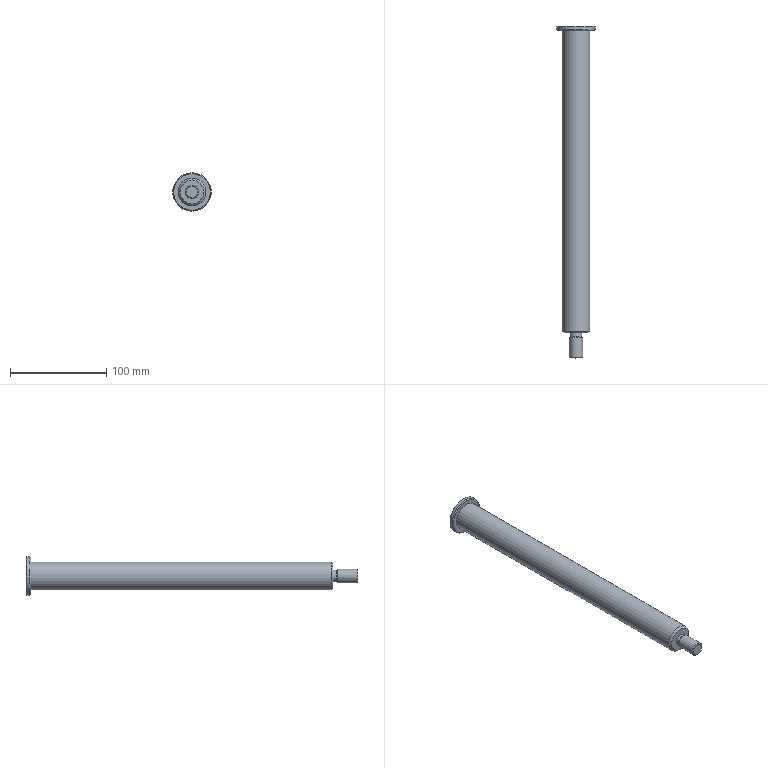Part | STEP file | HL4GZ-1.862.565 swing arm short shaft | 1 solid | 13 faces | box 40 x 345 x 40 mm | volume 217186 mm3 | cone 5 | plane 4 | cylinder 4 | commonest cylinder face diameters 12 x1 14 x1 29 x1 40 x1
STEP:
#1=CARTESIAN_POINT('',(0.,0.,0.));
#2=DIRECTION('',(0.,0.,1.));
#3=DIRECTION('',(1.,0.,0.));
#4=AXIS2_PLACEMENT_3D('',#1,#2,#3);
#5=CARTESIAN_POINT('',(1626.526,-17.,-146.534));
#6=VERTEX_POINT('',#5);
#7=CARTESIAN_POINT('',(1631.,-17.,-165.));
#8=DIRECTION('',(0.,-1.,0.));
#9=DIRECTION('',(0.2355,0.,-0.9719));
#10=AXIS2_PLACEMENT_3D('',#7,#8,#9);
#11=CIRCLE('',#10,19.);
#12=CARTESIAN_POINT('',(1631.,-17.,-165.));
#13=DIRECTION('',(0.,1.,0.));
#14=DIRECTION('',(-0.2355,0.,0.9719));
#15=AXIS2_PLACEMENT_3D('',#12,#13,#14);
#16=PLANE('',#15);
#17=CARTESIAN_POINT('',(-19.,0.));
#18=CARTESIAN_POINT('',(-19.,32.909));
#19=CARTESIAN_POINT('',(9.5,16.454));
#20=CARTESIAN_POINT('',(38.,0.));
#21=CARTESIAN_POINT('',(9.5,-16.454));
#22=CARTESIAN_POINT('',(-19.,-32.909));
#23=CARTESIAN_POINT('',(-19.,0.));
#24=(BOUNDED_CURVE()B_SPLINE_CURVE(2,(#17,#18,#19,#20,#21,#22,#23),.UNSPECIFIED.,.T.,.F.)B_SPLINE_CURVE_WITH_KNOTS((1,2,2,2,2,1),(-2.094,0.,2.094,4.189,6.283,8.378),.UNSPECIFIED.)CURVE()GEOMETRIC_REPRESENTATION_ITEM()RATIONAL_B_SPLINE_CURVE((1.,0.5,1.,0.5,1.,0.5,1.))REPRESENTATION_ITEM(''));
#25=(GEOMETRIC_REPRESENTATION_CONTEXT(2)PARAMETRIC_REPRESENTATION_CONTEXT()REPRESENTATION_CONTEXT('',''));
#26=DEFINITIONAL_REPRESENTATION('',(#24),#25);
#27=PCURVE('',#16,#26);
#28=CARTESIAN_POINT('',(1631.,-17.5,-165.));
#29=DIRECTION('',(0.,-1.,0.));
#30=DIRECTION('',(0.2355,0.,-0.9719));
#31=AXIS2_PLACEMENT_3D('',#28,#29,#30);
#32=CONICAL_SURFACE('',#31,19.5,0.7854);
#33=CARTESIAN_POINT('',(0.,-0.5));
#34=DIRECTION('',(1.,0.));
#35=VECTOR('',#34,1.);
#36=LINE('',#33,#35);
#37=(GEOMETRIC_REPRESENTATION_CONTEXT(2)PARAMETRIC_REPRESENTATION_CONTEXT()REPRESENTATION_CONTEXT('',''));
#38=DEFINITIONAL_REPRESENTATION('',(#36),#37);
#39=PCURVE('',#32,#38);
#40=SURFACE_CURVE('',#11,(#27,#39),.PCURVE_S1.);
#41=EDGE_CURVE('',#6,#6,#40,.T.);
#42=ORIENTED_EDGE('',*,*,#41,.F.);
#43=EDGE_LOOP('',(#42));
#44=FACE_BOUND('',#43,.T.);
#45=ADVANCED_FACE('',(#44),#16,.T.);
#46=ORIENTED_EDGE('',*,*,#41,.T.);
#47=CARTESIAN_POINT('',(1626.29,-18.,-145.562));
#48=VERTEX_POINT('',#47);
#49=CARTESIAN_POINT('',(1626.526,-17.,-146.534));
#50=CARTESIAN_POINT('',(1626.29,-18.,-145.562));
#51=B_SPLINE_CURVE_WITH_KNOTS('',1,(#49,#50),.UNSPECIFIED.,.F.,.F.,(2,2),(-0.7071,0.7071),.PIECEWISE_BEZIER_KNOTS.);
#52=CARTESIAN_POINT('',(9.425,0.));
#53=DIRECTION('',(0.,1.));
#54=VECTOR('',#53,1.);
#55=LINE('',#52,#54);
#56=(GEOMETRIC_REPRESENTATION_CONTEXT(2)PARAMETRIC_REPRESENTATION_CONTEXT()REPRESENTATION_CONTEXT('',''));
#57=DEFINITIONAL_REPRESENTATION('',(#55),#56);
#58=PCURVE('',#32,#57);
#59=CARTESIAN_POINT('',(3.142,0.));
#60=DIRECTION('',(0.,1.));
#61=VECTOR('',#60,1.);
#62=LINE('',#59,#61);
#63=(GEOMETRIC_REPRESENTATION_CONTEXT(2)PARAMETRIC_REPRESENTATION_CONTEXT()REPRESENTATION_CONTEXT('',''));
#64=DEFINITIONAL_REPRESENTATION('',(#62),#63);
#65=PCURVE('',#32,#64);
#66=SEAM_CURVE('',#51,(#58,#65),.PCURVE_S1.);
#67=EDGE_CURVE('',#6,#48,#66,.T.);
#68=ORIENTED_EDGE('',*,*,#67,.T.);
#69=CARTESIAN_POINT('',(1631.,-18.,-165.));
#70=DIRECTION('',(0.,1.,0.));
#71=DIRECTION('',(0.2355,0.,-0.9719));
#72=AXIS2_PLACEMENT_3D('',#69,#70,#71);
#73=CIRCLE('',#72,20.);
#74=CARTESIAN_POINT('',(12.566,0.5));
#75=DIRECTION('',(-1.,0.));
#76=VECTOR('',#75,1.);
#77=LINE('',#74,#76);
#78=(GEOMETRIC_REPRESENTATION_CONTEXT(2)PARAMETRIC_REPRESENTATION_CONTEXT()REPRESENTATION_CONTEXT('',''));
#79=DEFINITIONAL_REPRESENTATION('',(#77),#78);
#80=PCURVE('',#32,#79);
#81=CARTESIAN_POINT('',(1631.,-22.,-165.));
#82=DIRECTION('',(0.,1.,0.));
#83=DIRECTION('',(0.2355,0.,-0.9719));
#84=AXIS2_PLACEMENT_3D('',#81,#82,#83);
#85=CYLINDRICAL_SURFACE('',#84,20.);
#86=CARTESIAN_POINT('',(0.,4.));
#87=DIRECTION('',(1.,0.));
#88=VECTOR('',#87,1.);
#89=LINE('',#86,#88);
#90=(GEOMETRIC_REPRESENTATION_CONTEXT(2)PARAMETRIC_REPRESENTATION_CONTEXT()REPRESENTATION_CONTEXT('',''));
#91=DEFINITIONAL_REPRESENTATION('',(#89),#90);
#92=PCURVE('',#85,#91);
#93=SURFACE_CURVE('',#73,(#80,#92),.PCURVE_S1.);
#94=EDGE_CURVE('',#48,#48,#93,.T.);
#95=ORIENTED_EDGE('',*,*,#94,.T.);
#96=ORIENTED_EDGE('',*,*,#67,.F.);
#97=EDGE_LOOP('',(#46,#68,#95,#96));
#98=FACE_BOUND('',#97,.T.);
#99=ADVANCED_FACE('',(#98),#32,.T.);
#100=ORIENTED_EDGE('',*,*,#94,.F.);
#101=CARTESIAN_POINT('',(1626.29,-21.,-145.562));
#102=VERTEX_POINT('',#101);
#103=CARTESIAN_POINT('',(1626.29,-21.,-145.562));
#104=CARTESIAN_POINT('',(1626.29,-18.,-145.562));
#105=B_SPLINE_CURVE_WITH_KNOTS('',1,(#103,#104),.UNSPECIFIED.,.F.,.F.,(2,2),(1.,4.),.PIECEWISE_BEZIER_KNOTS.);
#106=CARTESIAN_POINT('',(3.142,0.));
#107=DIRECTION('',(0.,1.));
#108=VECTOR('',#107,1.);
#109=LINE('',#106,#108);
#110=(GEOMETRIC_REPRESENTATION_CONTEXT(2)PARAMETRIC_REPRESENTATION_CONTEXT()REPRESENTATION_CONTEXT('',''));
#111=DEFINITIONAL_REPRESENTATION('',(#109),#110);
#112=PCURVE('',#85,#111);
#113=CARTESIAN_POINT('',(9.425,0.));
#114=DIRECTION('',(0.,1.));
#115=VECTOR('',#114,1.);
#116=LINE('',#113,#115);
#117=(GEOMETRIC_REPRESENTATION_CONTEXT(2)PARAMETRIC_REPRESENTATION_CONTEXT()REPRESENTATION_CONTEXT('',''));
#118=DEFINITIONAL_REPRESENTATION('',(#116),#117);
#119=PCURVE('',#85,#118);
#120=SEAM_CURVE('',#105,(#112,#119),.PCURVE_S1.);
#121=EDGE_CURVE('',#102,#48,#120,.T.);
#122=ORIENTED_EDGE('',*,*,#121,.F.);
#123=CARTESIAN_POINT('',(1631.,-21.,-165.));
#124=DIRECTION('',(0.,-1.,0.));
#125=DIRECTION('',(0.2355,0.,-0.9719));
#126=AXIS2_PLACEMENT_3D('',#123,#124,#125);
#127=CIRCLE('',#126,20.);
#128=CARTESIAN_POINT('',(12.566,1.));
#129=DIRECTION('',(-1.,0.));
#130=VECTOR('',#129,1.);
#131=LINE('',#128,#130);
#132=(GEOMETRIC_REPRESENTATION_CONTEXT(2)PARAMETRIC_REPRESENTATION_CONTEXT()REPRESENTATION_CONTEXT('',''));
#133=DEFINITIONAL_REPRESENTATION('',(#131),#132);
#134=PCURVE('',#85,#133);
#135=CARTESIAN_POINT('',(1631.,-21.5,-165.));
#136=DIRECTION('',(0.,1.,0.));
#137=DIRECTION('',(0.2355,0.,-0.9719));
#138=AXIS2_PLACEMENT_3D('',#135,#136,#137);
#139=CONICAL_SURFACE('',#138,19.5,0.7854);
#140=CARTESIAN_POINT('',(12.566,0.5));
#141=DIRECTION('',(-1.,0.));
#142=VECTOR('',#141,1.);
#143=LINE('',#140,#142);
#144=(GEOMETRIC_REPRESENTATION_CONTEXT(2)PARAMETRIC_REPRESENTATION_CONTEXT()REPRESENTATION_CONTEXT('',''));
#145=DEFINITIONAL_REPRESENTATION('',(#143),#144);
#146=PCURVE('',#139,#145);
#147=SURFACE_CURVE('',#127,(#134,#146),.PCURVE_S1.);
#148=EDGE_CURVE('',#102,#102,#147,.T.);
#149=ORIENTED_EDGE('',*,*,#148,.F.);
#150=ORIENTED_EDGE('',*,*,#121,.T.);
#151=EDGE_LOOP('',(#100,#122,#149,#150));
#152=FACE_BOUND('',#151,.T.);
#153=ADVANCED_FACE('',(#152),#85,.T.);
#154=CARTESIAN_POINT('',(1626.526,-22.,-146.534));
#155=VERTEX_POINT('',#154);
#156=CARTESIAN_POINT('',(1631.,-22.,-165.));
#157=DIRECTION('',(0.,1.,0.));
#158=DIRECTION('',(0.2355,0.,-0.9719));
#159=AXIS2_PLACEMENT_3D('',#156,#157,#158);
#160=CIRCLE('',#159,19.);
#161=CARTESIAN_POINT('',(0.,-0.5));
#162=DIRECTION('',(1.,0.));
#163=VECTOR('',#162,1.);
#164=LINE('',#161,#163);
#165=(GEOMETRIC_REPRESENTATION_CONTEXT(2)PARAMETRIC_REPRESENTATION_CONTEXT()REPRESENTATION_CONTEXT('',''));
#166=DEFINITIONAL_REPRESENTATION('',(#164),#165);
#167=PCURVE('',#139,#166);
#168=CARTESIAN_POINT('',(1631.,-22.,-165.));
#169=DIRECTION('',(0.,1.,0.));
#170=DIRECTION('',(-0.2355,0.,0.9719));
#171=AXIS2_PLACEMENT_3D('',#168,#169,#170);
#172=PLANE('',#171);
#173=CARTESIAN_POINT('',(0.,0.));
#174=DIRECTION('',(-1.,0.));
#175=AXIS2_PLACEMENT_2D('',#173,#174);
#176=CIRCLE('',#175,19.);
#177=(GEOMETRIC_REPRESENTATION_CONTEXT(2)PARAMETRIC_REPRESENTATION_CONTEXT()REPRESENTATION_CONTEXT('',''));
#178=DEFINITIONAL_REPRESENTATION('',(#176),#177);
#179=PCURVE('',#172,#178);
#180=SURFACE_CURVE('',#160,(#167,#179),.PCURVE_S1.);
#181=EDGE_CURVE('',#155,#155,#180,.T.);
#182=ORIENTED_EDGE('',*,*,#181,.T.);
#183=CARTESIAN_POINT('',(1626.526,-22.,-146.534));
#184=CARTESIAN_POINT('',(1626.29,-21.,-145.562));
#185=B_SPLINE_CURVE_WITH_KNOTS('',1,(#183,#184),.UNSPECIFIED.,.F.,.F.,(2,2),(-0.7071,0.7071),.PIECEWISE_BEZIER_KNOTS.);
#186=CARTESIAN_POINT('',(9.425,0.));
#187=DIRECTION('',(0.,1.));
#188=VECTOR('',#187,1.);
#189=LINE('',#186,#188);
#190=(GEOMETRIC_REPRESENTATION_CONTEXT(2)PARAMETRIC_REPRESENTATION_CONTEXT()REPRESENTATION_CONTEXT('',''));
#191=DEFINITIONAL_REPRESENTATION('',(#189),#190);
#192=PCURVE('',#139,#191);
#193=CARTESIAN_POINT('',(3.142,0.));
#194=DIRECTION('',(0.,1.));
#195=VECTOR('',#194,1.);
#196=LINE('',#193,#195);
#197=(GEOMETRIC_REPRESENTATION_CONTEXT(2)PARAMETRIC_REPRESENTATION_CONTEXT()REPRESENTATION_CONTEXT('',''));
#198=DEFINITIONAL_REPRESENTATION('',(#196),#197);
#199=PCURVE('',#139,#198);
#200=SEAM_CURVE('',#185,(#192,#199),.PCURVE_S1.);
#201=EDGE_CURVE('',#155,#102,#200,.T.);
#202=ORIENTED_EDGE('',*,*,#201,.T.);
#203=ORIENTED_EDGE('',*,*,#148,.T.);
#204=ORIENTED_EDGE('',*,*,#201,.F.);
#205=EDGE_LOOP('',(#182,#202,#203,#204));
#206=FACE_BOUND('',#205,.T.);
#207=ADVANCED_FACE('',(#206),#139,.T.);
#208=CARTESIAN_POINT('',(1627.585,-22.,-150.908));
#209=VERTEX_POINT('',#208);
#210=CARTESIAN_POINT('',(1631.,-22.,-165.));
#211=DIRECTION('',(0.,-1.,0.));
#212=DIRECTION('',(0.2355,0.,-0.9719));
#213=AXIS2_PLACEMENT_3D('',#210,#211,#212);
#214=CIRCLE('',#213,14.5);
#215=CARTESIAN_POINT('',(-14.5,0.));
#216=CARTESIAN_POINT('',(-14.5,25.115));
#217=CARTESIAN_POINT('',(7.25,12.557));
#218=CARTESIAN_POINT('',(29.,0.));
#219=CARTESIAN_POINT('',(7.25,-12.557));
#220=CARTESIAN_POINT('',(-14.5,-25.115));
#221=CARTESIAN_POINT('',(-14.5,0.));
#222=(BOUNDED_CURVE()B_SPLINE_CURVE(2,(#215,#216,#217,#218,#219,#220,#221),.UNSPECIFIED.,.T.,.F.)B_SPLINE_CURVE_WITH_KNOTS((1,2,2,2,2,1),(-2.094,0.,2.094,4.189,6.283,8.378),.UNSPECIFIED.)CURVE()GEOMETRIC_REPRESENTATION_ITEM()RATIONAL_B_SPLINE_CURVE((1.,0.5,1.,0.5,1.,0.5,1.))REPRESENTATION_ITEM(''));
#223=(GEOMETRIC_REPRESENTATION_CONTEXT(2)PARAMETRIC_REPRESENTATION_CONTEXT()REPRESENTATION_CONTEXT('',''));
#224=DEFINITIONAL_REPRESENTATION('',(#222),#223);
#225=PCURVE('',#172,#224);
#226=CARTESIAN_POINT('',(1631.,-22.,-165.));
#227=DIRECTION('',(0.,-1.,0.));
#228=DIRECTION('',(0.2355,0.,-0.9719));
#229=AXIS2_PLACEMENT_3D('',#226,#227,#228);
#230=CYLINDRICAL_SURFACE('',#229,14.5);
#231=CARTESIAN_POINT('',(0.,0.));
#232=DIRECTION('',(1.,0.));
#233=VECTOR('',#232,1.);
#234=LINE('',#231,#233);
#235=(GEOMETRIC_REPRESENTATION_CONTEXT(2)PARAMETRIC_REPRESENTATION_CONTEXT()REPRESENTATION_CONTEXT('',''));
#236=DEFINITIONAL_REPRESENTATION('',(#234),#235);
#237=PCURVE('',#230,#236);
#238=SURFACE_CURVE('',#214,(#225,#237),.PCURVE_S1.);
#239=EDGE_CURVE('',#209,#209,#238,.T.);
#240=ORIENTED_EDGE('',*,*,#239,.F.);
#241=EDGE_LOOP('',(#240));
#242=FACE_BOUND('',#241,.T.);
#243=ORIENTED_EDGE('',*,*,#181,.F.);
#244=EDGE_LOOP('',(#243));
#245=FACE_BOUND('',#244,.T.);
#246=ADVANCED_FACE('',(#242,#245),#172,.F.);
#247=ORIENTED_EDGE('',*,*,#239,.T.);
#248=CARTESIAN_POINT('',(1627.585,-334.,-150.908));
#249=VERTEX_POINT('',#248);
#250=CARTESIAN_POINT('',(1627.585,-22.,-150.908));
#251=CARTESIAN_POINT('',(1627.585,-334.,-150.908));
#252=B_SPLINE_CURVE_WITH_KNOTS('',1,(#250,#251),.UNSPECIFIED.,.F.,.F.,(2,2),(0.,312.),.PIECEWISE_BEZIER_KNOTS.);
#253=CARTESIAN_POINT('',(9.425,0.));
#254=DIRECTION('',(0.,1.));
#255=VECTOR('',#254,1.);
#256=LINE('',#253,#255);
#257=(GEOMETRIC_REPRESENTATION_CONTEXT(2)PARAMETRIC_REPRESENTATION_CONTEXT()REPRESENTATION_CONTEXT('',''));
#258=DEFINITIONAL_REPRESENTATION('',(#256),#257);
#259=PCURVE('',#230,#258);
#260=CARTESIAN_POINT('',(3.142,0.));
#261=DIRECTION('',(0.,1.));
#262=VECTOR('',#261,1.);
#263=LINE('',#260,#262);
#264=(GEOMETRIC_REPRESENTATION_CONTEXT(2)PARAMETRIC_REPRESENTATION_CONTEXT()REPRESENTATION_CONTEXT('',''));
#265=DEFINITIONAL_REPRESENTATION('',(#263),#264);
#266=PCURVE('',#230,#265);
#267=SEAM_CURVE('',#252,(#259,#266),.PCURVE_S1.);
#268=EDGE_CURVE('',#209,#249,#267,.T.);
#269=ORIENTED_EDGE('',*,*,#268,.T.);
#270=CARTESIAN_POINT('',(1631.,-334.,-165.));
#271=DIRECTION('',(0.,-1.,0.));
#272=DIRECTION('',(0.2355,0.,-0.9719));
#273=AXIS2_PLACEMENT_3D('',#270,#271,#272);
#274=CIRCLE('',#273,14.5);
#275=CARTESIAN_POINT('',(0.,312.));
#276=DIRECTION('',(1.,0.));
#277=VECTOR('',#276,1.);
#278=LINE('',#275,#277);
#279=(GEOMETRIC_REPRESENTATION_CONTEXT(2)PARAMETRIC_REPRESENTATION_CONTEXT()REPRESENTATION_CONTEXT('',''));
#280=DEFINITIONAL_REPRESENTATION('',(#278),#279);
#281=PCURVE('',#230,#280);
#282=CARTESIAN_POINT('',(1631.,-335.,-165.));
#283=DIRECTION('',(0.,1.,0.));
#284=DIRECTION('',(0.2355,0.,-0.9719));
#285=AXIS2_PLACEMENT_3D('',#282,#283,#284);
#286=CONICAL_SURFACE('',#285,13.5,0.7854);
#287=CARTESIAN_POINT('',(12.566,1.));
#288=DIRECTION('',(-1.,0.));
#289=VECTOR('',#288,1.);
#290=LINE('',#287,#289);
#291=(GEOMETRIC_REPRESENTATION_CONTEXT(2)PARAMETRIC_REPRESENTATION_CONTEXT()REPRESENTATION_CONTEXT('',''));
#292=DEFINITIONAL_REPRESENTATION('',(#290),#291);
#293=PCURVE('',#286,#292);
#294=SURFACE_CURVE('',#274,(#281,#293),.PCURVE_S1.);
#295=EDGE_CURVE('',#249,#249,#294,.T.);
#296=ORIENTED_EDGE('',*,*,#295,.F.);
#297=ORIENTED_EDGE('',*,*,#268,.F.);
#298=EDGE_LOOP('',(#247,#269,#296,#297));
#299=FACE_BOUND('',#298,.T.);
#300=ADVANCED_FACE('',(#299),#230,.T.);
#301=CARTESIAN_POINT('',(1632.413,-362.,-170.831));
#302=VERTEX_POINT('',#301);
#303=CARTESIAN_POINT('',(1631.,-362.,-165.));
#304=DIRECTION('',(0.,1.,0.));
#305=DIRECTION('',(-0.2355,0.,0.9719));
#306=AXIS2_PLACEMENT_3D('',#303,#304,#305);
#307=CIRCLE('',#306,6.);
#308=CARTESIAN_POINT('',(1631.,-362.,-165.));
#309=DIRECTION('',(0.,1.,0.));
#310=DIRECTION('',(-0.2355,0.,0.9719));
#311=AXIS2_PLACEMENT_3D('',#308,#309,#310);
#312=PLANE('',#311);
#313=CARTESIAN_POINT('',(0.,0.));
#314=DIRECTION('',(1.,0.));
#315=AXIS2_PLACEMENT_2D('',#313,#314);
#316=CIRCLE('',#315,6.);
#317=(GEOMETRIC_REPRESENTATION_CONTEXT(2)PARAMETRIC_REPRESENTATION_CONTEXT()REPRESENTATION_CONTEXT('',''));
#318=DEFINITIONAL_REPRESENTATION('',(#316),#317);
#319=PCURVE('',#312,#318);
#320=CARTESIAN_POINT('',(1631.,-361.5,-165.));
#321=DIRECTION('',(0.,1.,0.));
#322=DIRECTION('',(-0.2355,0.,0.9719));
#323=AXIS2_PLACEMENT_3D('',#320,#321,#322);
#324=CONICAL_SURFACE('',#323,6.5,0.7854);
#325=CARTESIAN_POINT('',(0.,-0.5));
#326=DIRECTION('',(1.,0.));
#327=VECTOR('',#326,1.);
#328=LINE('',#325,#327);
#329=(GEOMETRIC_REPRESENTATION_CONTEXT(2)PARAMETRIC_REPRESENTATION_CONTEXT()REPRESENTATION_CONTEXT('',''));
#330=DEFINITIONAL_REPRESENTATION('',(#328),#329);
#331=PCURVE('',#324,#330);
#332=SURFACE_CURVE('',#307,(#319,#331),.PCURVE_S1.);
#333=EDGE_CURVE('',#302,#302,#332,.T.);
#334=ORIENTED_EDGE('',*,*,#333,.F.);
#335=EDGE_LOOP('',(#334));
#336=FACE_BOUND('',#335,.T.);
#337=ADVANCED_FACE('',(#336),#312,.F.);
#338=ORIENTED_EDGE('',*,*,#333,.T.);
#339=CARTESIAN_POINT('',(1632.648,-361.,-171.803));
#340=VERTEX_POINT('',#339);
#341=CARTESIAN_POINT('',(1632.413,-362.,-170.831));
#342=CARTESIAN_POINT('',(1632.648,-361.,-171.803));
#343=B_SPLINE_CURVE_WITH_KNOTS('',1,(#341,#342),.UNSPECIFIED.,.F.,.F.,(2,2),(-0.7071,0.7071),.PIECEWISE_BEZIER_KNOTS.);
#344=CARTESIAN_POINT('',(9.425,0.));
#345=DIRECTION('',(0.,1.));
#346=VECTOR('',#345,1.);
#347=LINE('',#344,#346);
#348=(GEOMETRIC_REPRESENTATION_CONTEXT(2)PARAMETRIC_REPRESENTATION_CONTEXT()REPRESENTATION_CONTEXT('',''));
#349=DEFINITIONAL_REPRESENTATION('',(#347),#348);
#350=PCURVE('',#324,#349);
#351=CARTESIAN_POINT('',(3.142,0.));
#352=DIRECTION('',(0.,1.));
#353=VECTOR('',#352,1.);
#354=LINE('',#351,#353);
#355=(GEOMETRIC_REPRESENTATION_CONTEXT(2)PARAMETRIC_REPRESENTATION_CONTEXT()REPRESENTATION_CONTEXT('',''));
#356=DEFINITIONAL_REPRESENTATION('',(#354),#355);
#357=PCURVE('',#324,#356);
#358=SEAM_CURVE('',#343,(#350,#357),.PCURVE_S1.);
#359=EDGE_CURVE('',#302,#340,#358,.T.);
#360=ORIENTED_EDGE('',*,*,#359,.T.);
#361=CARTESIAN_POINT('',(1631.,-361.,-165.));
#362=DIRECTION('',(0.,-1.,0.));
#363=DIRECTION('',(-0.2355,0.,0.9719));
#364=AXIS2_PLACEMENT_3D('',#361,#362,#363);
#365=CIRCLE('',#364,7.);
#366=CARTESIAN_POINT('',(12.566,0.5));
#367=DIRECTION('',(-1.,0.));
#368=VECTOR('',#367,1.);
#369=LINE('',#366,#368);
#370=(GEOMETRIC_REPRESENTATION_CONTEXT(2)PARAMETRIC_REPRESENTATION_CONTEXT()REPRESENTATION_CONTEXT('',''));
#371=DEFINITIONAL_REPRESENTATION('',(#369),#370);
#372=PCURVE('',#324,#371);
#373=CARTESIAN_POINT('',(1631.,-340.,-165.));
#374=DIRECTION('',(0.,-1.,0.));
#375=DIRECTION('',(-0.2355,0.,0.9719));
#376=AXIS2_PLACEMENT_3D('',#373,#374,#375);
#377=CYLINDRICAL_SURFACE('',#376,7.);
#378=CARTESIAN_POINT('',(0.,21.));
#379=DIRECTION('',(1.,0.));
#380=VECTOR('',#379,1.);
#381=LINE('',#378,#380);
#382=(GEOMETRIC_REPRESENTATION_CONTEXT(2)PARAMETRIC_REPRESENTATION_CONTEXT()REPRESENTATION_CONTEXT('',''));
#383=DEFINITIONAL_REPRESENTATION('',(#381),#382);
#384=PCURVE('',#377,#383);
#385=SURFACE_CURVE('',#365,(#372,#384),.PCURVE_S1.);
#386=EDGE_CURVE('',#340,#340,#385,.T.);
#387=ORIENTED_EDGE('',*,*,#386,.T.);
#388=ORIENTED_EDGE('',*,*,#359,.F.);
#389=EDGE_LOOP('',(#338,#360,#387,#388));
#390=FACE_BOUND('',#389,.T.);
#391=ADVANCED_FACE('',(#390),#324,.T.);
#392=ORIENTED_EDGE('',*,*,#386,.F.);
#393=CARTESIAN_POINT('',(1632.648,-341.,-171.803));
#394=VERTEX_POINT('',#393);
#395=CARTESIAN_POINT('',(1632.648,-341.,-171.803));
#396=CARTESIAN_POINT('',(1632.648,-361.,-171.803));
#397=B_SPLINE_CURVE_WITH_KNOTS('',1,(#395,#396),.UNSPECIFIED.,.F.,.F.,(2,2),(1.,21.),.PIECEWISE_BEZIER_KNOTS.);
#398=CARTESIAN_POINT('',(3.142,0.));
#399=DIRECTION('',(0.,1.));
#400=VECTOR('',#399,1.);
#401=LINE('',#398,#400);
#402=(GEOMETRIC_REPRESENTATION_CONTEXT(2)PARAMETRIC_REPRESENTATION_CONTEXT()REPRESENTATION_CONTEXT('',''));
#403=DEFINITIONAL_REPRESENTATION('',(#401),#402);
#404=PCURVE('',#377,#403);
#405=CARTESIAN_POINT('',(9.425,0.));
#406=DIRECTION('',(0.,1.));
#407=VECTOR('',#406,1.);
#408=LINE('',#405,#407);
#409=(GEOMETRIC_REPRESENTATION_CONTEXT(2)PARAMETRIC_REPRESENTATION_CONTEXT()REPRESENTATION_CONTEXT('',''));
#410=DEFINITIONAL_REPRESENTATION('',(#408),#409);
#411=PCURVE('',#377,#410);
#412=SEAM_CURVE('',#397,(#404,#411),.PCURVE_S1.);
#413=EDGE_CURVE('',#394,#340,#412,.T.);
#414=ORIENTED_EDGE('',*,*,#413,.F.);
#415=CARTESIAN_POINT('',(1631.,-341.,-165.));
#416=DIRECTION('',(0.,1.,0.));
#417=DIRECTION('',(-0.2355,0.,0.9719));
#418=AXIS2_PLACEMENT_3D('',#415,#416,#417);
#419=CIRCLE('',#418,7.);
#420=CARTESIAN_POINT('',(12.566,1.));
#421=DIRECTION('',(-1.,0.));
#422=VECTOR('',#421,1.);
#423=LINE('',#420,#422);
#424=(GEOMETRIC_REPRESENTATION_CONTEXT(2)PARAMETRIC_REPRESENTATION_CONTEXT()REPRESENTATION_CONTEXT('',''));
#425=DEFINITIONAL_REPRESENTATION('',(#423),#424);
#426=PCURVE('',#377,#425);
#427=CARTESIAN_POINT('',(1631.,-340.5,-165.));
#428=DIRECTION('',(0.,-1.,0.));
#429=DIRECTION('',(-0.2355,0.,0.9719));
#430=AXIS2_PLACEMENT_3D('',#427,#428,#429);
#431=CONICAL_SURFACE('',#430,6.5,0.7854);
#432=CARTESIAN_POINT('',(12.566,0.5));
#433=DIRECTION('',(-1.,0.));
#434=VECTOR('',#433,1.);
#435=LINE('',#432,#434);
#436=(GEOMETRIC_REPRESENTATION_CONTEXT(2)PARAMETRIC_REPRESENTATION_CONTEXT()REPRESENTATION_CONTEXT('',''));
#437=DEFINITIONAL_REPRESENTATION('',(#435),#436);
#438=PCURVE('',#431,#437);
#439=SURFACE_CURVE('',#419,(#426,#438),.PCURVE_S1.);
#440=EDGE_CURVE('',#394,#394,#439,.T.);
#441=ORIENTED_EDGE('',*,*,#440,.F.);
#442=ORIENTED_EDGE('',*,*,#413,.T.);
#443=EDGE_LOOP('',(#392,#414,#441,#442));
#444=FACE_BOUND('',#443,.T.);
#445=ADVANCED_FACE('',(#444),#377,.T.);
#446=CARTESIAN_POINT('',(1632.413,-340.,-170.831));
#447=VERTEX_POINT('',#446);
#448=CARTESIAN_POINT('',(1631.,-340.,-165.));
#449=DIRECTION('',(0.,-1.,0.));
#450=DIRECTION('',(-0.2355,0.,0.9719));
#451=AXIS2_PLACEMENT_3D('',#448,#449,#450);
#452=CIRCLE('',#451,6.);
#453=CARTESIAN_POINT('',(0.,-0.5));
#454=DIRECTION('',(1.,0.));
#455=VECTOR('',#454,1.);
#456=LINE('',#453,#455);
#457=(GEOMETRIC_REPRESENTATION_CONTEXT(2)PARAMETRIC_REPRESENTATION_CONTEXT()REPRESENTATION_CONTEXT('',''));
#458=DEFINITIONAL_REPRESENTATION('',(#456),#457);
#459=PCURVE('',#431,#458);
#460=CARTESIAN_POINT('',(1631.,-336.,-165.));
#461=DIRECTION('',(0.,-1.,0.));
#462=DIRECTION('',(-0.2355,0.,0.9719));
#463=AXIS2_PLACEMENT_3D('',#460,#461,#462);
#464=CYLINDRICAL_SURFACE('',#463,6.);
#465=CARTESIAN_POINT('',(0.,4.));
#466=DIRECTION('',(1.,0.));
#467=VECTOR('',#466,1.);
#468=LINE('',#465,#467);
#469=(GEOMETRIC_REPRESENTATION_CONTEXT(2)PARAMETRIC_REPRESENTATION_CONTEXT()REPRESENTATION_CONTEXT('',''));
#470=DEFINITIONAL_REPRESENTATION('',(#468),#469);
#471=PCURVE('',#464,#470);
#472=SURFACE_CURVE('',#452,(#459,#471),.PCURVE_S1.);
#473=EDGE_CURVE('',#447,#447,#472,.T.);
#474=ORIENTED_EDGE('',*,*,#473,.T.);
#475=CARTESIAN_POINT('',(1632.413,-340.,-170.831));
#476=CARTESIAN_POINT('',(1632.648,-341.,-171.803));
#477=B_SPLINE_CURVE_WITH_KNOTS('',1,(#475,#476),.UNSPECIFIED.,.F.,.F.,(2,2),(-0.7071,0.7071),.PIECEWISE_BEZIER_KNOTS.);
#478=CARTESIAN_POINT('',(9.425,0.));
#479=DIRECTION('',(0.,1.));
#480=VECTOR('',#479,1.);
#481=LINE('',#478,#480);
#482=(GEOMETRIC_REPRESENTATION_CONTEXT(2)PARAMETRIC_REPRESENTATION_CONTEXT()REPRESENTATION_CONTEXT('',''));
#483=DEFINITIONAL_REPRESENTATION('',(#481),#482);
#484=PCURVE('',#431,#483);
#485=CARTESIAN_POINT('',(3.142,0.));
#486=DIRECTION('',(0.,1.));
#487=VECTOR('',#486,1.);
#488=LINE('',#485,#487);
#489=(GEOMETRIC_REPRESENTATION_CONTEXT(2)PARAMETRIC_REPRESENTATION_CONTEXT()REPRESENTATION_CONTEXT('',''));
#490=DEFINITIONAL_REPRESENTATION('',(#488),#489);
#491=PCURVE('',#431,#490);
#492=SEAM_CURVE('',#477,(#484,#491),.PCURVE_S1.);
#493=EDGE_CURVE('',#447,#394,#492,.T.);
#494=ORIENTED_EDGE('',*,*,#493,.T.);
#495=ORIENTED_EDGE('',*,*,#440,.T.);
#496=ORIENTED_EDGE('',*,*,#493,.F.);
#497=EDGE_LOOP('',(#474,#494,#495,#496));
#498=FACE_BOUND('',#497,.T.);
#499=ADVANCED_FACE('',(#498),#431,.T.);
#500=CARTESIAN_POINT('',(1632.413,-336.,-170.831));
#501=VERTEX_POINT('',#500);
#502=CARTESIAN_POINT('',(1631.,-336.,-165.));
#503=DIRECTION('',(0.,1.,0.));
#504=DIRECTION('',(-0.2355,0.,0.9719));
#505=AXIS2_PLACEMENT_3D('',#502,#503,#504);
#506=CIRCLE('',#505,6.);
#507=CARTESIAN_POINT('',(12.566,0.));
#508=DIRECTION('',(-1.,0.));
#509=VECTOR('',#508,1.);
#510=LINE('',#507,#509);
#511=(GEOMETRIC_REPRESENTATION_CONTEXT(2)PARAMETRIC_REPRESENTATION_CONTEXT()REPRESENTATION_CONTEXT('',''));
#512=DEFINITIONAL_REPRESENTATION('',(#510),#511);
#513=PCURVE('',#464,#512);
#514=CARTESIAN_POINT('',(1631.,-336.,-165.));
#515=DIRECTION('',(0.,1.,0.));
#516=DIRECTION('',(-0.2355,0.,0.9719));
#517=AXIS2_PLACEMENT_3D('',#514,#515,#516);
#518=PLANE('',#517);
#519=CARTESIAN_POINT('',(0.,0.));
#520=DIRECTION('',(1.,0.));
#521=AXIS2_PLACEMENT_2D('',#519,#520);
#522=CIRCLE('',#521,6.);
#523=(GEOMETRIC_REPRESENTATION_CONTEXT(2)PARAMETRIC_REPRESENTATION_CONTEXT()REPRESENTATION_CONTEXT('',''));
#524=DEFINITIONAL_REPRESENTATION('',(#522),#523);
#525=PCURVE('',#518,#524);
#526=SURFACE_CURVE('',#506,(#513,#525),.PCURVE_S1.);
#527=EDGE_CURVE('',#501,#501,#526,.T.);
#528=ORIENTED_EDGE('',*,*,#527,.F.);
#529=CARTESIAN_POINT('',(1632.413,-336.,-170.831));
#530=CARTESIAN_POINT('',(1632.413,-340.,-170.831));
#531=B_SPLINE_CURVE_WITH_KNOTS('',1,(#529,#530),.UNSPECIFIED.,.F.,.F.,(2,2),(0.,4.),.PIECEWISE_BEZIER_KNOTS.);
#532=CARTESIAN_POINT('',(9.425,0.));
#533=DIRECTION('',(0.,1.));
#534=VECTOR('',#533,1.);
#535=LINE('',#532,#534);
#536=(GEOMETRIC_REPRESENTATION_CONTEXT(2)PARAMETRIC_REPRESENTATION_CONTEXT()REPRESENTATION_CONTEXT('',''));
#537=DEFINITIONAL_REPRESENTATION('',(#535),#536);
#538=PCURVE('',#464,#537);
#539=CARTESIAN_POINT('',(3.142,0.));
#540=DIRECTION('',(0.,1.));
#541=VECTOR('',#540,1.);
#542=LINE('',#539,#541);
#543=(GEOMETRIC_REPRESENTATION_CONTEXT(2)PARAMETRIC_REPRESENTATION_CONTEXT()REPRESENTATION_CONTEXT('',''));
#544=DEFINITIONAL_REPRESENTATION('',(#542),#543);
#545=PCURVE('',#464,#544);
#546=SEAM_CURVE('',#531,(#538,#545),.PCURVE_S1.);
#547=EDGE_CURVE('',#501,#447,#546,.T.);
#548=ORIENTED_EDGE('',*,*,#547,.T.);
#549=ORIENTED_EDGE('',*,*,#473,.F.);
#550=ORIENTED_EDGE('',*,*,#547,.F.);
#551=EDGE_LOOP('',(#528,#548,#549,#550));
#552=FACE_BOUND('',#551,.T.);
#553=ADVANCED_FACE('',(#552),#464,.T.);
#554=ORIENTED_EDGE('',*,*,#527,.T.);
#555=EDGE_LOOP('',(#554));
#556=FACE_BOUND('',#555,.T.);
#557=CARTESIAN_POINT('',(1628.056,-336.,-152.852));
#558=VERTEX_POINT('',#557);
#559=CARTESIAN_POINT('',(1631.,-336.,-165.));
#560=DIRECTION('',(0.,1.,0.));
#561=DIRECTION('',(0.2355,0.,-0.9719));
#562=AXIS2_PLACEMENT_3D('',#559,#560,#561);
#563=CIRCLE('',#562,12.5);
#564=CARTESIAN_POINT('',(0.,0.));
#565=DIRECTION('',(-1.,0.));
#566=AXIS2_PLACEMENT_2D('',#564,#565);
#567=CIRCLE('',#566,12.5);
#568=(GEOMETRIC_REPRESENTATION_CONTEXT(2)PARAMETRIC_REPRESENTATION_CONTEXT()REPRESENTATION_CONTEXT('',''));
#569=DEFINITIONAL_REPRESENTATION('',(#567),#568);
#570=PCURVE('',#518,#569);
#571=CARTESIAN_POINT('',(0.,-1.));
#572=DIRECTION('',(1.,0.));
#573=VECTOR('',#572,1.);
#574=LINE('',#571,#573);
#575=(GEOMETRIC_REPRESENTATION_CONTEXT(2)PARAMETRIC_REPRESENTATION_CONTEXT()REPRESENTATION_CONTEXT('',''));
#576=DEFINITIONAL_REPRESENTATION('',(#574),#575);
#577=PCURVE('',#286,#576);
#578=SURFACE_CURVE('',#563,(#570,#577),.PCURVE_S1.);
#579=EDGE_CURVE('',#558,#558,#578,.T.);
#580=ORIENTED_EDGE('',*,*,#579,.F.);
#581=EDGE_LOOP('',(#580));
#582=FACE_BOUND('',#581,.T.);
#583=ADVANCED_FACE('',(#556,#582),#518,.F.);
#584=ORIENTED_EDGE('',*,*,#579,.T.);
#585=CARTESIAN_POINT('',(1628.056,-336.,-152.852));
#586=CARTESIAN_POINT('',(1627.585,-334.,-150.908));
#587=B_SPLINE_CURVE_WITH_KNOTS('',1,(#585,#586),.UNSPECIFIED.,.F.,.F.,(2,2),(-1.414,1.414),.PIECEWISE_BEZIER_KNOTS.);
#588=CARTESIAN_POINT('',(9.425,0.));
#589=DIRECTION('',(0.,1.));
#590=VECTOR('',#589,1.);
#591=LINE('',#588,#590);
#592=(GEOMETRIC_REPRESENTATION_CONTEXT(2)PARAMETRIC_REPRESENTATION_CONTEXT()REPRESENTATION_CONTEXT('',''));
#593=DEFINITIONAL_REPRESENTATION('',(#591),#592);
#594=PCURVE('',#286,#593);
#595=CARTESIAN_POINT('',(3.142,0.));
#596=DIRECTION('',(0.,1.));
#597=VECTOR('',#596,1.);
#598=LINE('',#595,#597);
#599=(GEOMETRIC_REPRESENTATION_CONTEXT(2)PARAMETRIC_REPRESENTATION_CONTEXT()REPRESENTATION_CONTEXT('',''));
#600=DEFINITIONAL_REPRESENTATION('',(#598),#599);
#601=PCURVE('',#286,#600);
#602=SEAM_CURVE('',#587,(#594,#601),.PCURVE_S1.);
#603=EDGE_CURVE('',#558,#249,#602,.T.);
#604=ORIENTED_EDGE('',*,*,#603,.T.);
#605=ORIENTED_EDGE('',*,*,#295,.T.);
#606=ORIENTED_EDGE('',*,*,#603,.F.);
#607=EDGE_LOOP('',(#584,#604,#605,#606));
#608=FACE_BOUND('',#607,.T.);
#609=ADVANCED_FACE('',(#608),#286,.T.);
#610=CLOSED_SHELL('',(#45,#99,#153,#207,#246,#300,#337,#391,#445,#499,#553,#583,#609));
#611=MANIFOLD_SOLID_BREP('',#610);
#612=(LENGTH_UNIT()NAMED_UNIT(*)SI_UNIT(.MILLI.,.METRE.));
#613=UNCERTAINTY_MEASURE_WITH_UNIT(LENGTH_MEASURE(0.00001),#612,'','');
#614=(NAMED_UNIT(*)PLANE_ANGLE_UNIT()SI_UNIT($,.RADIAN.));
#615=(NAMED_UNIT(*)SI_UNIT($,.STERADIAN.)SOLID_ANGLE_UNIT());
#616=(GEOMETRIC_REPRESENTATION_CONTEXT(3)GLOBAL_UNCERTAINTY_ASSIGNED_CONTEXT((#613))GLOBAL_UNIT_ASSIGNED_CONTEXT((#612,#614,#615))REPRESENTATION_CONTEXT('',''));
#617=ADVANCED_BREP_SHAPE_REPRESENTATION('',(#4,#611),#616);